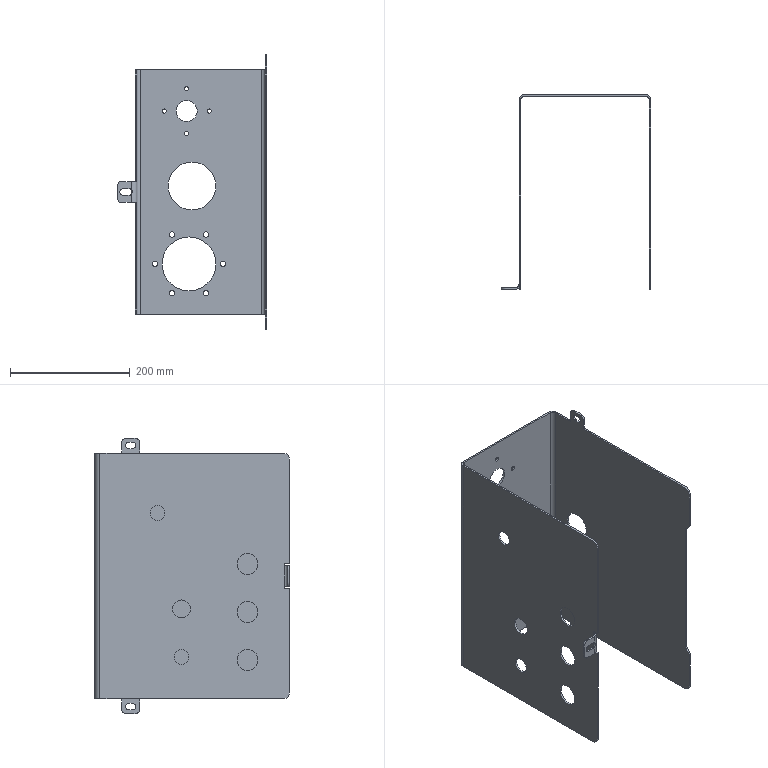Part | SolidWorks | features ICE 8, Fillet 5, EdgeFlange 1, FlatPattern 1, SMBaseFlange 1, SheetMetal 1 | 1 solid | 117 faces | box 250 x 325 x 460 mm | volume 996726 mm3 | cylinder 70 | plane 46 | spline 1 | commonest cylinder face diameters 9 x12 7 x8 11 x8 35 x8 15 x6 20 x6